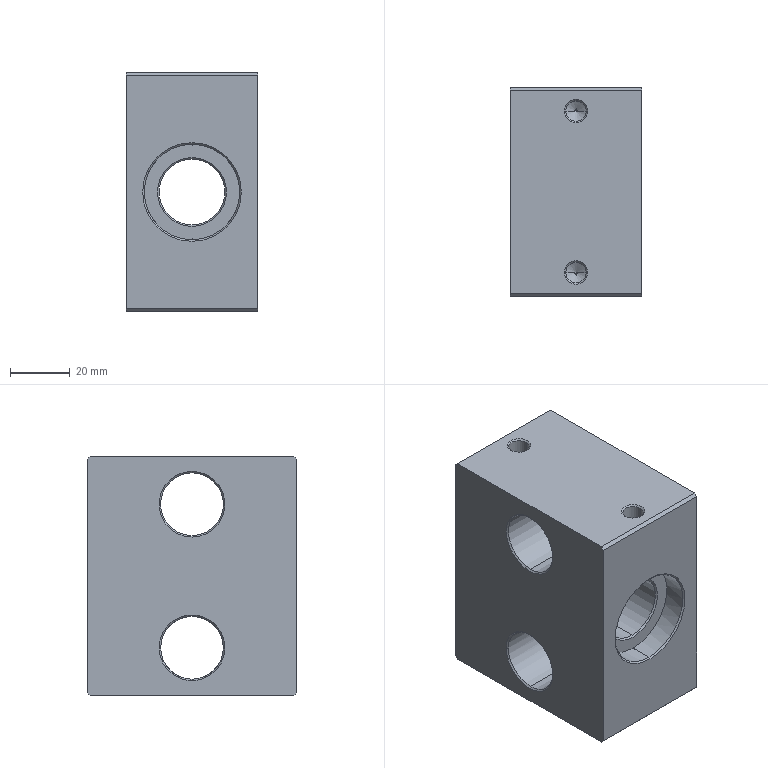Part | STEP file | longitudinal seal bearing seat 2_SUS304 | 1 solid | 86 faces | box 44 x 70 x 80 mm | volume 178257 mm3 | cone 44 | cylinder 30 | plane 12 | commonest cylinder face diameters 3.3 x12 6.8 x8 21 x4 32 x4 22 x2